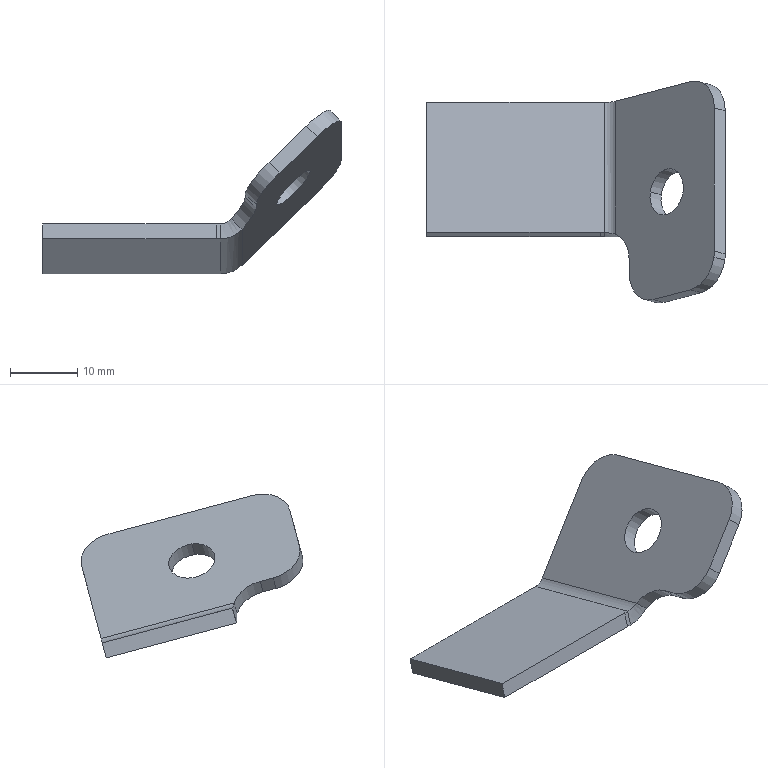Part | SolidWorks | features BaseBody 1, FlatPattern 1, SheetMetal 1, SolidToSheetMetal 1 | 1 solid | 23 faces | box 44.304 x 32.939 x 24.3 mm | volume 2673 mm3 | plane 12 | cylinder 9 | spline 2 | commonest cylinder face diameters 10 x5 7 x2 4.6 x1 9.2 x1
STEP:
#1=CARTESIAN_POINT('',(1147.365,61.574,741.478));
#2=VERTEX_POINT('',#1);
#3=CARTESIAN_POINT('',(1142.501,61.574,736.443));
#4=VERTEX_POINT('',#3);
#5=CARTESIAN_POINT('',(1144.933,61.574,738.961));
#6=DIRECTION('',(0.7071,-0.183,-0.683));
#7=DIRECTION('',(-0.6947,0.,-0.7193));
#8=AXIS2_PLACEMENT_3D('',#5,#6,#7);
#9=CIRCLE('',#8,3.5);
#10=EDGE_CURVE('',#2,#4,#9,.T.);
#11=ORIENTED_EDGE('',*,*,#10,.T.);
#12=CARTESIAN_POINT('',(1140.875,61.995,738.014));
#13=VERTEX_POINT('',#12);
#14=CARTESIAN_POINT('',(1140.875,61.995,738.014));
#15=DIRECTION('',(-0.7071,0.183,0.683));
#16=VECTOR('',#15,1000.);
#17=LINE('',#14,#16);
#18=EDGE_CURVE('',#4,#13,#17,.T.);
#19=ORIENTED_EDGE('',*,*,#18,.T.);
#20=CARTESIAN_POINT('',(1145.738,61.995,743.049));
#21=VERTEX_POINT('',#20);
#22=CARTESIAN_POINT('',(1143.307,61.995,740.532));
#23=DIRECTION('',(0.7071,-0.183,-0.683));
#24=DIRECTION('',(-0.6947,0.,-0.7193));
#25=AXIS2_PLACEMENT_3D('',#22,#23,#24);
#26=CIRCLE('',#25,3.5);
#27=EDGE_CURVE('',#21,#13,#26,.T.);
#28=ORIENTED_EDGE('',*,*,#27,.F.);
#29=CARTESIAN_POINT('',(1145.738,61.995,743.049));
#30=DIRECTION('',(-0.7071,0.183,0.683));
#31=VECTOR('',#30,1000.);
#32=LINE('',#29,#31);
#33=EDGE_CURVE('',#2,#21,#32,.T.);
#34=ORIENTED_EDGE('',*,*,#33,.F.);
#35=EDGE_LOOP('',(#11,#19,#28,#34));
#36=FACE_OUTER_BOUND('',#35,.T.);
#37=CARTESIAN_POINT('',(1143.307,61.995,740.532));
#38=DIRECTION('',(-0.7071,0.183,0.683));
#39=DIRECTION('',(0.6947,0.,0.7193));
#40=AXIS2_PLACEMENT_3D('',#37,#38,#39);
#41=CYLINDRICAL_SURFACE('',#40,3.5);
#42=ADVANCED_FACE('',(#36),#41,.F.);
#43=CARTESIAN_POINT('',(1148.468,47.034,746.517));
#44=VERTEX_POINT('',#43);
#45=CARTESIAN_POINT('',(1151.942,51.864,748.819));
#46=VERTEX_POINT('',#45);
#47=CARTESIAN_POINT('',(1148.468,51.864,745.223));
#48=DIRECTION('',(-0.7071,0.183,0.683));
#49=DIRECTION('',(-0.6947,0.,-0.7193));
#50=AXIS2_PLACEMENT_3D('',#47,#48,#49);
#51=CIRCLE('',#50,5.);
#52=EDGE_CURVE('',#44,#46,#51,.T.);
#53=ORIENTED_EDGE('',*,*,#52,.T.);
#54=CARTESIAN_POINT('',(1150.316,52.285,750.39));
#55=VERTEX_POINT('',#54);
#56=CARTESIAN_POINT('',(1150.316,52.285,750.39));
#57=DIRECTION('',(-0.7071,0.183,0.683));
#58=VECTOR('',#57,1000.);
#59=LINE('',#56,#58);
#60=EDGE_CURVE('',#46,#55,#59,.T.);
#61=ORIENTED_EDGE('',*,*,#60,.T.);
#62=CARTESIAN_POINT('',(1146.842,47.455,748.088));
#63=VERTEX_POINT('',#62);
#64=CARTESIAN_POINT('',(1146.842,52.285,746.794));
#65=DIRECTION('',(-0.7071,0.183,0.683));
#66=DIRECTION('',(-0.6947,0.,-0.7193));
#67=AXIS2_PLACEMENT_3D('',#64,#65,#66);
#68=CIRCLE('',#67,5.);
#69=EDGE_CURVE('',#63,#55,#68,.T.);
#70=ORIENTED_EDGE('',*,*,#69,.F.);
#71=CARTESIAN_POINT('',(1146.842,47.455,748.088));
#72=DIRECTION('',(-0.7071,0.183,0.683));
#73=VECTOR('',#72,1000.);
#74=LINE('',#71,#73);
#75=EDGE_CURVE('',#44,#63,#74,.T.);
#76=ORIENTED_EDGE('',*,*,#75,.F.);
#77=EDGE_LOOP('',(#53,#61,#70,#76));
#78=FACE_OUTER_BOUND('',#77,.T.);
#79=CARTESIAN_POINT('',(1146.842,52.285,746.794));
#80=DIRECTION('',(-0.7071,0.183,0.683));
#81=DIRECTION('',(0.6947,0.,0.7193));
#82=AXIS2_PLACEMENT_3D('',#79,#80,#81);
#83=CYLINDRICAL_SURFACE('',#82,5.);
#84=ADVANCED_FACE('',(#78),#83,.T.);
#85=CARTESIAN_POINT('',(1139.381,51.444,735.927));
#86=VERTEX_POINT('',#85);
#87=CARTESIAN_POINT('',(1137.755,51.865,737.498));
#88=VERTEX_POINT('',#87);
#89=CARTESIAN_POINT('',(1137.755,51.865,737.498));
#90=DIRECTION('',(-0.7071,0.183,0.683));
#91=VECTOR('',#90,1000.);
#92=LINE('',#89,#91);
#93=EDGE_CURVE('',#86,#88,#92,.T.);
#94=ORIENTED_EDGE('',*,*,#93,.F.);
#95=CARTESIAN_POINT('',(1139.381,49.512,736.445));
#96=VERTEX_POINT('',#95);
#97=CARTESIAN_POINT('',(1139.381,51.444,735.927));
#98=DIRECTION('',(-0.000000007,-0.9659,0.2588));
#99=VECTOR('',#98,1000.);
#100=LINE('',#97,#99);
#101=EDGE_CURVE('',#86,#96,#100,.T.);
#102=ORIENTED_EDGE('',*,*,#101,.T.);
#103=CARTESIAN_POINT('',(1137.755,49.933,738.016));
#104=VERTEX_POINT('',#103);
#105=CARTESIAN_POINT('',(1137.755,49.933,738.016));
#106=DIRECTION('',(-0.7071,0.183,0.683));
#107=VECTOR('',#106,1000.);
#108=LINE('',#105,#107);
#109=EDGE_CURVE('',#96,#104,#108,.T.);
#110=ORIENTED_EDGE('',*,*,#109,.T.);
#111=CARTESIAN_POINT('',(1137.755,51.865,737.498));
#112=DIRECTION('',(-0.000000007,-0.9659,0.2588));
#113=VECTOR('',#112,1000.);
#114=LINE('',#111,#113);
#115=EDGE_CURVE('',#88,#104,#114,.T.);
#116=ORIENTED_EDGE('',*,*,#115,.F.);
#117=EDGE_LOOP('',(#94,#102,#110,#116));
#118=FACE_OUTER_BOUND('',#117,.T.);
#119=CARTESIAN_POINT('',(1137.755,51.865,737.498));
#120=DIRECTION('',(-0.7071,-0.183,-0.683));
#121=DIRECTION('',(-0.000000007,-0.9659,0.2588));
#122=AXIS2_PLACEMENT_3D('',#119,#120,#121);
#123=PLANE('',#122);
#124=ADVANCED_FACE('',(#118),#123,.T.);
#125=ORIENTED_EDGE('',*,*,#109,.F.);
#126=CARTESIAN_POINT('',(1142.917,45.597,741.154));
#127=VERTEX_POINT('',#126);
#128=CARTESIAN_POINT('',(1142.917,50.427,739.86));
#129=DIRECTION('',(-0.7071,0.183,0.683));
#130=DIRECTION('',(0.6947,0.,0.7193));
#131=AXIS2_PLACEMENT_3D('',#128,#129,#130);
#132=CIRCLE('',#131,5.);
#133=EDGE_CURVE('',#96,#127,#132,.T.);
#134=ORIENTED_EDGE('',*,*,#133,.T.);
#135=CARTESIAN_POINT('',(1141.29,46.018,742.725));
#136=VERTEX_POINT('',#135);
#137=CARTESIAN_POINT('',(1141.29,46.018,742.725));
#138=DIRECTION('',(-0.7071,0.183,0.683));
#139=VECTOR('',#138,1000.);
#140=LINE('',#137,#139);
#141=EDGE_CURVE('',#127,#136,#140,.T.);
#142=ORIENTED_EDGE('',*,*,#141,.T.);
#143=CARTESIAN_POINT('',(1141.29,50.848,741.431));
#144=DIRECTION('',(-0.7071,0.183,0.683));
#145=DIRECTION('',(0.6947,0.,0.7193));
#146=AXIS2_PLACEMENT_3D('',#143,#144,#145);
#147=CIRCLE('',#146,5.);
#148=EDGE_CURVE('',#104,#136,#147,.T.);
#149=ORIENTED_EDGE('',*,*,#148,.F.);
#150=EDGE_LOOP('',(#125,#134,#142,#149));
#151=FACE_OUTER_BOUND('',#150,.T.);
#152=CARTESIAN_POINT('',(1141.29,50.848,741.431));
#153=DIRECTION('',(-0.7071,0.183,0.683));
#154=DIRECTION('',(0.6947,0.,0.7193));
#155=AXIS2_PLACEMENT_3D('',#152,#153,#154);
#156=CYLINDRICAL_SURFACE('',#155,5.);
#157=ADVANCED_FACE('',(#151),#156,.T.);
#158=ORIENTED_EDGE('',*,*,#141,.F.);
#159=CARTESIAN_POINT('',(1142.917,45.597,741.154));
#160=DIRECTION('',(0.7071,0.183,0.683));
#161=VECTOR('',#160,1000.);
#162=LINE('',#159,#161);
#163=EDGE_CURVE('',#127,#44,#162,.T.);
#164=ORIENTED_EDGE('',*,*,#163,.T.);
#165=ORIENTED_EDGE('',*,*,#75,.T.);
#166=CARTESIAN_POINT('',(1141.29,46.018,742.725));
#167=DIRECTION('',(0.7071,0.183,0.683));
#168=VECTOR('',#167,1000.);
#169=LINE('',#166,#168);
#170=EDGE_CURVE('',#136,#63,#169,.T.);
#171=ORIENTED_EDGE('',*,*,#170,.F.);
#172=EDGE_LOOP('',(#158,#164,#165,#171));
#173=FACE_OUTER_BOUND('',#172,.T.);
#174=CARTESIAN_POINT('',(1141.29,46.018,742.725));
#175=DIRECTION('',(0.000000002,-0.9659,0.2588));
#176=DIRECTION('',(0.7071,0.183,0.683));
#177=AXIS2_PLACEMENT_3D('',#174,#175,#176);
#178=PLANE('',#177);
#179=ADVANCED_FACE('',(#173),#178,.T.);
#180=ORIENTED_EDGE('',*,*,#60,.F.);
#181=CARTESIAN_POINT('',(1152.004,52.779,748.638));
#182=VERTEX_POINT('',#181);
#183=CARTESIAN_POINT('',(1148.468,51.864,745.223));
#184=DIRECTION('',(-0.7071,0.183,0.683));
#185=DIRECTION('',(-0.6947,0.,-0.7193));
#186=AXIS2_PLACEMENT_3D('',#183,#184,#185);
#187=CIRCLE('',#186,5.);
#188=EDGE_CURVE('',#46,#182,#187,.T.);
#189=ORIENTED_EDGE('',*,*,#188,.T.);
#190=CARTESIAN_POINT('',(1150.378,53.2,750.209));
#191=VERTEX_POINT('',#190);
#192=CARTESIAN_POINT('',(1150.378,53.2,750.209));
#193=DIRECTION('',(-0.7071,0.183,0.683));
#194=VECTOR('',#193,1000.);
#195=LINE('',#192,#194);
#196=EDGE_CURVE('',#182,#191,#195,.T.);
#197=ORIENTED_EDGE('',*,*,#196,.T.);
#198=CARTESIAN_POINT('',(1146.842,52.285,746.794));
#199=DIRECTION('',(-0.7071,0.183,0.683));
#200=DIRECTION('',(-0.6947,0.,-0.7193));
#201=AXIS2_PLACEMENT_3D('',#198,#199,#200);
#202=CIRCLE('',#201,5.);
#203=EDGE_CURVE('',#55,#191,#202,.T.);
#204=ORIENTED_EDGE('',*,*,#203,.F.);
#205=EDGE_LOOP('',(#180,#189,#197,#204));
#206=FACE_OUTER_BOUND('',#205,.T.);
#207=CARTESIAN_POINT('',(1146.842,52.285,746.794));
#208=DIRECTION('',(-0.7071,0.183,0.683));
#209=DIRECTION('',(0.6947,0.,0.7193));
#210=AXIS2_PLACEMENT_3D('',#207,#208,#209);
#211=CYLINDRICAL_SURFACE('',#210,5.);
#212=ADVANCED_FACE('',(#206),#211,.T.);
#213=ORIENTED_EDGE('',*,*,#196,.F.);
#214=CARTESIAN_POINT('',(1152.004,74.029,742.944));
#215=VERTEX_POINT('',#214);
#216=CARTESIAN_POINT('',(1152.004,52.779,748.638));
#217=DIRECTION('',(0.,0.9659,-0.2588));
#218=VECTOR('',#217,1000.);
#219=LINE('',#216,#218);
#220=EDGE_CURVE('',#182,#215,#219,.T.);
#221=ORIENTED_EDGE('',*,*,#220,.T.);
#222=CARTESIAN_POINT('',(1150.378,74.45,744.515));
#223=VERTEX_POINT('',#222);
#224=CARTESIAN_POINT('',(1150.378,74.45,744.515));
#225=DIRECTION('',(-0.7071,0.183,0.683));
#226=VECTOR('',#225,1000.);
#227=LINE('',#224,#226);
#228=EDGE_CURVE('',#215,#223,#227,.T.);
#229=ORIENTED_EDGE('',*,*,#228,.T.);
#230=CARTESIAN_POINT('',(1150.378,53.2,750.209));
#231=DIRECTION('',(0.,0.9659,-0.2588));
#232=VECTOR('',#231,1000.);
#233=LINE('',#230,#232);
#234=EDGE_CURVE('',#191,#223,#233,.T.);
#235=ORIENTED_EDGE('',*,*,#234,.F.);
#236=EDGE_LOOP('',(#213,#221,#229,#235));
#237=FACE_OUTER_BOUND('',#236,.T.);
#238=CARTESIAN_POINT('',(1150.378,53.2,750.209));
#239=DIRECTION('',(0.7071,0.183,0.683));
#240=DIRECTION('',(0.,0.9659,-0.2588));
#241=AXIS2_PLACEMENT_3D('',#238,#239,#240);
#242=PLANE('',#241);
#243=ADVANCED_FACE('',(#237),#242,.T.);
#244=ORIENTED_EDGE('',*,*,#228,.F.);
#245=CARTESIAN_POINT('',(1148.468,77.944,738.235));
#246=VERTEX_POINT('',#245);
#247=CARTESIAN_POINT('',(1148.468,73.114,739.529));
#248=DIRECTION('',(-0.7071,0.183,0.683));
#249=DIRECTION('',(-0.6947,0.,-0.7193));
#250=AXIS2_PLACEMENT_3D('',#247,#248,#249);
#251=CIRCLE('',#250,5.);
#252=EDGE_CURVE('',#215,#246,#251,.T.);
#253=ORIENTED_EDGE('',*,*,#252,.T.);
#254=CARTESIAN_POINT('',(1146.842,78.365,739.805));
#255=VERTEX_POINT('',#254);
#256=CARTESIAN_POINT('',(1146.842,78.365,739.805));
#257=DIRECTION('',(-0.7071,0.183,0.683));
#258=VECTOR('',#257,1000.);
#259=LINE('',#256,#258);
#260=EDGE_CURVE('',#246,#255,#259,.T.);
#261=ORIENTED_EDGE('',*,*,#260,.T.);
#262=CARTESIAN_POINT('',(1146.842,73.535,741.1));
#263=DIRECTION('',(-0.7071,0.183,0.683));
#264=DIRECTION('',(-0.6947,0.,-0.7193));
#265=AXIS2_PLACEMENT_3D('',#262,#263,#264);
#266=CIRCLE('',#265,5.);
#267=EDGE_CURVE('',#223,#255,#266,.T.);
#268=ORIENTED_EDGE('',*,*,#267,.F.);
#269=EDGE_LOOP('',(#244,#253,#261,#268));
#270=FACE_OUTER_BOUND('',#269,.T.);
#271=CARTESIAN_POINT('',(1146.842,73.535,741.1));
#272=DIRECTION('',(-0.7071,0.183,0.683));
#273=DIRECTION('',(0.6947,0.,0.7193));
#274=AXIS2_PLACEMENT_3D('',#271,#272,#273);
#275=CYLINDRICAL_SURFACE('',#274,5.);
#276=ADVANCED_FACE('',(#270),#275,.T.);
#277=ORIENTED_EDGE('',*,*,#260,.F.);
#278=CARTESIAN_POINT('',(1137.3,75.053,727.447));
#279=VERTEX_POINT('',#278);
#280=CARTESIAN_POINT('',(1148.468,77.944,738.235));
#281=DIRECTION('',(-0.7071,-0.183,-0.683));
#282=VECTOR('',#281,1000.);
#283=LINE('',#280,#282);
#284=EDGE_CURVE('',#246,#279,#283,.T.);
#285=ORIENTED_EDGE('',*,*,#284,.T.);
#286=CARTESIAN_POINT('',(1135.674,75.474,729.018));
#287=VERTEX_POINT('',#286);
#288=CARTESIAN_POINT('',(1135.674,75.474,729.018));
#289=DIRECTION('',(-0.7071,0.183,0.683));
#290=VECTOR('',#289,1000.);
#291=LINE('',#288,#290);
#292=EDGE_CURVE('',#279,#287,#291,.T.);
#293=ORIENTED_EDGE('',*,*,#292,.T.);
#294=CARTESIAN_POINT('',(1146.842,78.365,739.805));
#295=DIRECTION('',(-0.7071,-0.183,-0.683));
#296=VECTOR('',#295,1000.);
#297=LINE('',#294,#296);
#298=EDGE_CURVE('',#255,#287,#297,.T.);
#299=ORIENTED_EDGE('',*,*,#298,.F.);
#300=EDGE_LOOP('',(#277,#285,#293,#299));
#301=FACE_OUTER_BOUND('',#300,.T.);
#302=CARTESIAN_POINT('',(1146.842,78.365,739.805));
#303=DIRECTION('',(0.,0.9659,-0.2588));
#304=DIRECTION('',(-0.7071,-0.183,-0.683));
#305=AXIS2_PLACEMENT_3D('',#302,#303,#304);
#306=PLANE('',#305);
#307=ADVANCED_FACE('',(#301),#306,.T.);
#308=ORIENTED_EDGE('',*,*,#292,.F.);
#309=CARTESIAN_POINT('',(1134.047,74.705,726.145));
#310=VERTEX_POINT('',#309);
#311=CARTESIAN_POINT('',(1134.047,75.895,730.588));
#312=DIRECTION('',(0.,0.9659,-0.2588));
#313=DIRECTION('',(0.,0.2588,0.9659));
#314=AXIS2_PLACEMENT_3D('',#311,#312,#313);
#315=CIRCLE('',#314,4.6);
#316=EDGE_CURVE('',#279,#310,#315,.T.);
#317=ORIENTED_EDGE('',*,*,#316,.T.);
#318=CARTESIAN_POINT('',(1134.047,75.3,728.367));
#319=VERTEX_POINT('',#318);
#320=CARTESIAN_POINT('',(1134.047,75.3,728.367));
#321=DIRECTION('',(0.,0.2588,0.9659));
#322=VECTOR('',#321,1000.);
#323=LINE('',#320,#322);
#324=EDGE_CURVE('',#310,#319,#323,.T.);
#325=ORIENTED_EDGE('',*,*,#324,.T.);
#326=CARTESIAN_POINT('',(1134.047,75.895,730.588));
#327=DIRECTION('',(0.,0.9659,-0.2588));
#328=DIRECTION('',(0.,0.2588,0.9659));
#329=AXIS2_PLACEMENT_3D('',#326,#327,#328);
#330=CIRCLE('',#329,2.3);
#331=EDGE_CURVE('',#287,#319,#330,.T.);
#332=ORIENTED_EDGE('',*,*,#331,.F.);
#333=EDGE_LOOP('',(#308,#317,#325,#332));
#334=FACE_OUTER_BOUND('',#333,.T.);
#335=CARTESIAN_POINT('',(1134.047,75.895,730.588));
#336=DIRECTION('',(0.,-0.9659,0.2588));
#337=DIRECTION('',(0.,-0.2588,-0.9659));
#338=AXIS2_PLACEMENT_3D('',#335,#336,#337);
#339=PLANE('',#338);
#340=ADVANCED_FACE('',(#334),#339,.F.);
#341=ORIENTED_EDGE('',*,*,#324,.F.);
#342=CARTESIAN_POINT('',(1107.7,74.705,726.145));
#343=VERTEX_POINT('',#342);
#344=CARTESIAN_POINT('',(1134.047,74.705,726.145));
#345=DIRECTION('',(1.,0.,0.));
#346=VECTOR('',#345,1000.);
#347=LINE('',#344,#346);
#348=EDGE_CURVE('',#343,#310,#347,.T.);
#349=ORIENTED_EDGE('',*,*,#348,.F.);
#350=CARTESIAN_POINT('',(1107.7,75.3,728.367));
#351=VERTEX_POINT('',#350);
#352=CARTESIAN_POINT('',(1107.7,75.3,728.367));
#353=DIRECTION('',(0.,0.2588,0.9659));
#354=VECTOR('',#353,1000.);
#355=LINE('',#352,#354);
#356=EDGE_CURVE('',#343,#351,#355,.T.);
#357=ORIENTED_EDGE('',*,*,#356,.T.);
#358=CARTESIAN_POINT('',(1120.874,75.3,728.367));
#359=DIRECTION('',(1.,0.,0.));
#360=VECTOR('',#359,1000.);
#361=LINE('',#358,#360);
#362=EDGE_CURVE('',#351,#319,#361,.T.);
#363=ORIENTED_EDGE('',*,*,#362,.T.);
#364=EDGE_LOOP('',(#341,#349,#357,#363));
#365=FACE_OUTER_BOUND('',#364,.T.);
#366=CARTESIAN_POINT('',(1120.874,75.3,728.367));
#367=DIRECTION('',(0.,0.9659,-0.2588));
#368=DIRECTION('',(1.,0.,0.));
#369=AXIS2_PLACEMENT_3D('',#366,#367,#368);
#370=PLANE('',#369);
#371=ADVANCED_FACE('',(#365),#370,.T.);
#372=ORIENTED_EDGE('',*,*,#356,.F.);
#373=CARTESIAN_POINT('',(1107.7,55.386,731.322));
#374=VERTEX_POINT('',#373);
#375=CARTESIAN_POINT('',(1107.7,74.705,726.145));
#376=DIRECTION('',(0.,0.9659,-0.2588));
#377=VECTOR('',#376,1000.);
#378=LINE('',#375,#377);
#379=EDGE_CURVE('',#374,#343,#378,.T.);
#380=ORIENTED_EDGE('',*,*,#379,.F.);
#381=CARTESIAN_POINT('',(1107.7,55.981,733.543));
#382=VERTEX_POINT('',#381);
#383=CARTESIAN_POINT('',(1107.7,55.981,733.543));
#384=DIRECTION('',(0.,0.2588,0.9659));
#385=VECTOR('',#384,1000.);
#386=LINE('',#383,#385);
#387=EDGE_CURVE('',#374,#382,#386,.T.);
#388=ORIENTED_EDGE('',*,*,#387,.T.);
#389=CARTESIAN_POINT('',(1107.7,65.574,730.973));
#390=DIRECTION('',(0.,0.9659,-0.2588));
#391=VECTOR('',#390,1000.);
#392=LINE('',#389,#391);
#393=EDGE_CURVE('',#382,#351,#392,.T.);
#394=ORIENTED_EDGE('',*,*,#393,.T.);
#395=EDGE_LOOP('',(#372,#380,#388,#394));
#396=FACE_OUTER_BOUND('',#395,.T.);
#397=CARTESIAN_POINT('',(1107.7,65.574,730.973));
#398=DIRECTION('',(-1.,0.,0.));
#399=DIRECTION('',(0.,0.9659,-0.2588));
#400=AXIS2_PLACEMENT_3D('',#397,#398,#399);
#401=PLANE('',#400);
#402=ADVANCED_FACE('',(#396),#401,.T.);
#403=ORIENTED_EDGE('',*,*,#387,.F.);
#404=CARTESIAN_POINT('',(1133.438,55.386,731.322));
#405=VERTEX_POINT('',#404);
#406=CARTESIAN_POINT('',(1134.047,55.386,731.322));
#407=DIRECTION('',(-1.,0.,0.));
#408=VECTOR('',#407,1000.);
#409=LINE('',#406,#408);
#410=EDGE_CURVE('',#405,#374,#409,.T.);
#411=ORIENTED_EDGE('',*,*,#410,.F.);
#412=CARTESIAN_POINT('',(1133.438,55.981,733.543));
#413=VERTEX_POINT('',#412);
#414=CARTESIAN_POINT('',(1133.438,55.981,733.543));
#415=DIRECTION('',(0.,0.2588,0.9659));
#416=VECTOR('',#415,1000.);
#417=LINE('',#414,#416);
#418=EDGE_CURVE('',#405,#413,#417,.T.);
#419=ORIENTED_EDGE('',*,*,#418,.T.);
#420=CARTESIAN_POINT('',(1120.874,55.981,733.543));
#421=DIRECTION('',(-1.,0.,0.));
#422=VECTOR('',#421,1000.);
#423=LINE('',#420,#422);
#424=EDGE_CURVE('',#413,#382,#423,.T.);
#425=ORIENTED_EDGE('',*,*,#424,.T.);
#426=EDGE_LOOP('',(#403,#411,#419,#425));
#427=FACE_OUTER_BOUND('',#426,.T.);
#428=CARTESIAN_POINT('',(1120.874,55.981,733.543));
#429=DIRECTION('',(0.,-0.9659,0.2588));
#430=DIRECTION('',(-1.,0.,0.));
#431=AXIS2_PLACEMENT_3D('',#428,#429,#430);
#432=PLANE('',#431);
#433=ADVANCED_FACE('',(#427),#432,.T.);
#434=ORIENTED_EDGE('',*,*,#418,.F.);
#435=CARTESIAN_POINT('',(1134.047,55.368,731.326));
#436=VERTEX_POINT('',#435);
#437=CARTESIAN_POINT('',(1134.047,55.368,731.326));
#438=CARTESIAN_POINT('',(1133.845,55.38,731.323));
#439=CARTESIAN_POINT('',(1133.642,55.386,731.322));
#440=CARTESIAN_POINT('',(1133.438,55.386,731.322));
#441=(BOUNDED_CURVE()B_SPLINE_CURVE(3,(#437,#438,#439,#440),.UNSPECIFIED.,.F.,.F.)B_SPLINE_CURVE_WITH_KNOTS((4,4),(1.485,1.571),.UNSPECIFIED.)CURVE()GEOMETRIC_REPRESENTATION_ITEM()RATIONAL_B_SPLINE_CURVE((1.,0.9994,0.9994,1.))REPRESENTATION_ITEM(''));
#442=EDGE_CURVE('',#436,#405,#441,.T.);
#443=ORIENTED_EDGE('',*,*,#442,.F.);
#444=CARTESIAN_POINT('',(1134.047,55.964,733.548));
#445=VERTEX_POINT('',#444);
#446=CARTESIAN_POINT('',(1134.047,55.368,731.326));
#447=CARTESIAN_POINT('',(1134.047,55.964,733.548));
#448=B_SPLINE_CURVE_WITH_KNOTS('',1,(#446,#447),.UNSPECIFIED.,.F.,.F.,(2,2),(0.,1.),.UNSPECIFIED.);
#449=EDGE_CURVE('',#436,#445,#448,.T.);
#450=ORIENTED_EDGE('',*,*,#449,.T.);
#451=CARTESIAN_POINT('',(1134.047,55.964,733.548));
#452=CARTESIAN_POINT('',(1133.845,55.975,733.545));
#453=CARTESIAN_POINT('',(1133.642,55.981,733.543));
#454=CARTESIAN_POINT('',(1133.438,55.981,733.543));
#455=(BOUNDED_CURVE()B_SPLINE_CURVE(3,(#451,#452,#453,#454),.UNSPECIFIED.,.F.,.F.)B_SPLINE_CURVE_WITH_KNOTS((4,4),(1.485,1.571),.UNSPECIFIED.)CURVE()GEOMETRIC_REPRESENTATION_ITEM()RATIONAL_B_SPLINE_CURVE((1.,0.9994,0.9994,1.))REPRESENTATION_ITEM(''));
#456=EDGE_CURVE('',#445,#413,#455,.T.);
#457=ORIENTED_EDGE('',*,*,#456,.T.);
#458=EDGE_LOOP('',(#434,#443,#450,#457));
#459=FACE_OUTER_BOUND('',#458,.T.);
#460=CARTESIAN_POINT('',(1134.047,55.964,733.548));
#461=CARTESIAN_POINT('',(1134.047,55.368,731.326));
#462=CARTESIAN_POINT('',(1133.845,55.975,733.545));
#463=CARTESIAN_POINT('',(1133.845,55.38,731.323));
#464=CARTESIAN_POINT('',(1133.642,55.981,733.543));
#465=CARTESIAN_POINT('',(1133.642,55.386,731.322));
#466=CARTESIAN_POINT('',(1133.438,55.981,733.543));
#467=CARTESIAN_POINT('',(1133.438,55.386,731.322));
#468=(BOUNDED_SURFACE()B_SPLINE_SURFACE(3,1,((#460,#461),(#462,#463),(#464,#465),(#466,#467)),.UNSPECIFIED.,.F.,.F.,.F.)B_SPLINE_SURFACE_WITH_KNOTS((4,4),(2,2),(0.,1.),(0.,1.),.UNSPECIFIED.)GEOMETRIC_REPRESENTATION_ITEM()RATIONAL_B_SPLINE_SURFACE(((1.,1.),(0.9994,0.9994),(0.9994,0.9994),(1.,1.)))REPRESENTATION_ITEM('')SURFACE());
#469=ADVANCED_FACE('',(#459),#468,.F.);
#470=ORIENTED_EDGE('',*,*,#449,.F.);
#471=CARTESIAN_POINT('',(1137.3,55.307,732.738));
#472=VERTEX_POINT('',#471);
#473=CARTESIAN_POINT('',(1134.047,55.368,731.326));
#474=CARTESIAN_POINT('',(1134.36,55.359,731.329));
#475=CARTESIAN_POINT('',(1134.667,55.354,731.363));
#476=CARTESIAN_POINT('',(1135.268,55.346,731.492));
#477=CARTESIAN_POINT('',(1135.566,55.344,731.589));
#478=CARTESIAN_POINT('',(1136.122,55.338,731.835));
#479=CARTESIAN_POINT('',(1136.384,55.335,731.984));
#480=CARTESIAN_POINT('',(1136.873,55.324,732.33));
#481=CARTESIAN_POINT('',(1137.099,55.317,732.527));
#482=CARTESIAN_POINT('',(1137.3,55.307,732.738));
#483=B_SPLINE_CURVE_WITH_KNOTS('',3,(#473,#474,#475,#476,#477,#478,#479,#480,#481,#482),.UNSPECIFIED.,.F.,.F.,(4,2,2,2,4),(0.,0.25,0.5,0.75,1.),.UNSPECIFIED.);
#484=EDGE_CURVE('',#436,#472,#483,.T.);
#485=ORIENTED_EDGE('',*,*,#484,.T.);
#486=CARTESIAN_POINT('',(1135.674,55.728,734.308));
#487=VERTEX_POINT('',#486);
#488=CARTESIAN_POINT('',(1137.3,55.307,732.738));
#489=CARTESIAN_POINT('',(1135.674,55.728,734.308));
#490=B_SPLINE_CURVE_WITH_KNOTS('',1,(#488,#489),.UNSPECIFIED.,.F.,.F.,(2,2),(0.,1.),.UNSPECIFIED.);
#491=EDGE_CURVE('',#472,#487,#490,.T.);
#492=ORIENTED_EDGE('',*,*,#491,.T.);
#493=CARTESIAN_POINT('',(1134.047,55.964,733.548));
#494=CARTESIAN_POINT('',(1134.215,55.954,733.551));
#495=CARTESIAN_POINT('',(1134.376,55.943,733.573));
#496=CARTESIAN_POINT('',(1134.602,55.925,733.627));
#497=CARTESIAN_POINT('',(1134.675,55.919,733.649));
#498=CARTESIAN_POINT('',(1134.779,55.908,733.686));
#499=CARTESIAN_POINT('',(1134.831,55.903,733.706));
#500=CARTESIAN_POINT('',(1134.881,55.897,733.728));
#501=CARTESIAN_POINT('',(1134.913,55.893,733.742));
#502=CARTESIAN_POINT('',(1134.928,55.891,733.749));
#503=CARTESIAN_POINT('',(1135.223,55.853,733.889));
#504=CARTESIAN_POINT('',(1135.47,55.801,734.079));
#505=CARTESIAN_POINT('',(1135.674,55.728,734.308));
#506=B_SPLINE_CURVE_WITH_KNOTS('',3,(#493,#494,#495,#496,#497,#498,#499,#500,#501,#502,#503,#504,#505),.UNSPECIFIED.,.F.,.F.,(4,2,2,1,2,2,4),(0.,0.25,0.375,0.4375,0.4687,0.5,1.),.UNSPECIFIED.);
#507=EDGE_CURVE('',#445,#487,#506,.T.);
#508=ORIENTED_EDGE('',*,*,#507,.F.);
#509=EDGE_LOOP('',(#470,#485,#492,#508));
#510=FACE_OUTER_BOUND('',#509,.T.);
#511=CARTESIAN_POINT('',(1134.047,55.368,731.326));
#512=CARTESIAN_POINT('',(1134.36,55.359,731.329));
#513=CARTESIAN_POINT('',(1134.667,55.354,731.363));
#514=CARTESIAN_POINT('',(1135.268,55.346,731.492));
#515=CARTESIAN_POINT('',(1135.566,55.344,731.589));
#516=CARTESIAN_POINT('',(1136.122,55.338,731.835));
#517=CARTESIAN_POINT('',(1136.384,55.335,731.984));
#518=CARTESIAN_POINT('',(1136.873,55.324,732.33));
#519=CARTESIAN_POINT('',(1137.099,55.317,732.527));
#520=CARTESIAN_POINT('',(1137.3,55.307,732.738));
#521=CARTESIAN_POINT('',(1134.047,55.964,733.548));
#522=CARTESIAN_POINT('',(1134.204,55.954,733.551));
#523=CARTESIAN_POINT('',(1134.357,55.945,733.569));
#524=CARTESIAN_POINT('',(1134.658,55.921,733.639));
#525=CARTESIAN_POINT('',(1134.806,55.907,733.691));
#526=CARTESIAN_POINT('',(1135.085,55.871,733.823));
#527=CARTESIAN_POINT('',(1135.215,55.849,733.903));
#528=CARTESIAN_POINT('',(1135.46,55.796,734.089));
#529=CARTESIAN_POINT('',(1135.573,55.764,734.195));
#530=CARTESIAN_POINT('',(1135.674,55.728,734.308));
#531=B_SPLINE_SURFACE_WITH_KNOTS('',1,3,((#511,#512,#513,#514,#515,#516,#517,#518,#519,#520),(#521,#522,#523,#524,#525,#526,#527,#528,#529,#530)),.UNSPECIFIED.,.F.,.F.,.F.,(2,2),(4,2,2,2,4),(0.,1.),(0.,0.0004637,0.0009275,0.001391,0.001855),.UNSPECIFIED.);
#532=ADVANCED_FACE('',(#510),#531,.F.);
#533=ORIENTED_EDGE('',*,*,#18,.F.);
#534=CARTESIAN_POINT('',(1144.933,61.574,738.961));
#535=DIRECTION('',(0.7071,-0.183,-0.683));
#536=DIRECTION('',(-0.6947,0.,-0.7193));
#537=AXIS2_PLACEMENT_3D('',#534,#535,#536);
#538=CIRCLE('',#537,3.5);
#539=EDGE_CURVE('',#4,#2,#538,.T.);
#540=ORIENTED_EDGE('',*,*,#539,.T.);
#541=ORIENTED_EDGE('',*,*,#33,.T.);
#542=CARTESIAN_POINT('',(1143.307,61.995,740.532));
#543=DIRECTION('',(0.7071,-0.183,-0.683));
#544=DIRECTION('',(-0.6947,0.,-0.7193));
#545=AXIS2_PLACEMENT_3D('',#542,#543,#544);
#546=CIRCLE('',#545,3.5);
#547=EDGE_CURVE('',#13,#21,#546,.T.);
#548=ORIENTED_EDGE('',*,*,#547,.F.);
#549=EDGE_LOOP('',(#533,#540,#541,#548));
#550=FACE_OUTER_BOUND('',#549,.T.);
#551=CARTESIAN_POINT('',(1143.307,61.995,740.532));
#552=DIRECTION('',(-0.7071,0.183,0.683));
#553=DIRECTION('',(0.6947,0.,0.7193));
#554=AXIS2_PLACEMENT_3D('',#551,#552,#553);
#555=CYLINDRICAL_SURFACE('',#554,3.5);
#556=ADVANCED_FACE('',(#550),#555,.F.);
#557=CARTESIAN_POINT('',(1135.846,50.529,732.512));
#558=DIRECTION('',(0.7071,-0.183,-0.683));
#559=DIRECTION('',(-0.6947,0.,-0.7193));
#560=AXIS2_PLACEMENT_3D('',#557,#558,#559);
#561=CIRCLE('',#560,5.);
#562=EDGE_CURVE('',#472,#86,#561,.T.);
#563=ORIENTED_EDGE('',*,*,#562,.T.);
#564=ORIENTED_EDGE('',*,*,#93,.T.);
#565=CARTESIAN_POINT('',(1134.219,50.95,734.083));
#566=DIRECTION('',(0.7071,-0.183,-0.683));
#567=DIRECTION('',(-0.6947,0.,-0.7193));
#568=AXIS2_PLACEMENT_3D('',#565,#566,#567);
#569=CIRCLE('',#568,5.);
#570=EDGE_CURVE('',#487,#88,#569,.T.);
#571=ORIENTED_EDGE('',*,*,#570,.F.);
#572=ORIENTED_EDGE('',*,*,#491,.F.);
#573=EDGE_LOOP('',(#563,#564,#571,#572));
#574=FACE_OUTER_BOUND('',#573,.T.);
#575=CARTESIAN_POINT('',(1134.219,50.95,734.083));
#576=DIRECTION('',(-0.7071,0.183,0.683));
#577=DIRECTION('',(0.6947,0.,0.7193));
#578=AXIS2_PLACEMENT_3D('',#575,#576,#577);
#579=CYLINDRICAL_SURFACE('',#578,5.);
#580=ADVANCED_FACE('',(#574),#579,.F.);
#581=ORIENTED_EDGE('',*,*,#507,.T.);
#582=CARTESIAN_POINT('',(1135.674,65.542,731.679));
#583=DIRECTION('',(0.,0.9659,-0.2588));
#584=VECTOR('',#583,1000.);
#585=LINE('',#582,#584);
#586=EDGE_CURVE('',#487,#287,#585,.T.);
#587=ORIENTED_EDGE('',*,*,#586,.T.);
#588=ORIENTED_EDGE('',*,*,#331,.T.);
#589=CARTESIAN_POINT('',(1134.047,65.574,730.973));
#590=DIRECTION('',(0.,-0.9659,0.2588));
#591=VECTOR('',#590,1000.);
#592=LINE('',#589,#591);
#593=EDGE_CURVE('',#319,#445,#592,.T.);
#594=ORIENTED_EDGE('',*,*,#593,.T.);
#595=EDGE_LOOP('',(#581,#587,#588,#594));
#596=FACE_OUTER_BOUND('',#595,.T.);
#597=CARTESIAN_POINT('',(1134.047,56.031,735.911));
#598=DIRECTION('',(0.,0.9659,-0.2588));
#599=DIRECTION('',(0.,0.2588,0.9659));
#600=AXIS2_PLACEMENT_3D('',#597,#598,#599);
#601=CYLINDRICAL_SURFACE('',#600,2.3);
#602=ADVANCED_FACE('',(#596),#601,.F.);
#603=ORIENTED_EDGE('',*,*,#593,.F.);
#604=ORIENTED_EDGE('',*,*,#362,.F.);
#605=ORIENTED_EDGE('',*,*,#393,.F.);
#606=ORIENTED_EDGE('',*,*,#424,.F.);
#607=ORIENTED_EDGE('',*,*,#456,.F.);
#608=EDGE_LOOP('',(#603,#604,#605,#606,#607));
#609=FACE_OUTER_BOUND('',#608,.T.);
#610=CARTESIAN_POINT('',(1134.047,75.3,728.367));
#611=DIRECTION('',(0.,-0.2588,-0.9659));
#612=DIRECTION('',(0.,-0.9659,0.2588));
#613=AXIS2_PLACEMENT_3D('',#610,#611,#612);
#614=PLANE('',#613);
#615=ADVANCED_FACE('',(#609),#614,.F.);
#616=ORIENTED_EDGE('',*,*,#27,.T.);
#617=ORIENTED_EDGE('',*,*,#547,.T.);
#618=EDGE_LOOP('',(#616,#617));
#619=FACE_BOUND('',#618,.T.);
#620=ORIENTED_EDGE('',*,*,#570,.T.);
#621=ORIENTED_EDGE('',*,*,#115,.T.);
#622=ORIENTED_EDGE('',*,*,#148,.T.);
#623=ORIENTED_EDGE('',*,*,#170,.T.);
#624=ORIENTED_EDGE('',*,*,#69,.T.);
#625=ORIENTED_EDGE('',*,*,#203,.T.);
#626=ORIENTED_EDGE('',*,*,#234,.T.);
#627=ORIENTED_EDGE('',*,*,#267,.T.);
#628=ORIENTED_EDGE('',*,*,#298,.T.);
#629=ORIENTED_EDGE('',*,*,#586,.F.);
#630=EDGE_LOOP('',(#620,#621,#622,#623,#624,#625,#626,#627,#628,#629));
#631=FACE_OUTER_BOUND('',#630,.T.);
#632=CARTESIAN_POINT('',(1148.265,43.671,750.574));
#633=DIRECTION('',(-0.7071,0.183,0.683));
#634=DIRECTION('',(0.2506,0.9681,0.));
#635=AXIS2_PLACEMENT_3D('',#632,#633,#634);
#636=PLANE('',#635);
#637=ADVANCED_FACE('',(#619,#631),#636,.T.);
#638=ORIENTED_EDGE('',*,*,#484,.F.);
#639=CARTESIAN_POINT('',(1134.047,74.705,726.145));
#640=DIRECTION('',(0.,-0.9659,0.2588));
#641=VECTOR('',#640,1000.);
#642=LINE('',#639,#641);
#643=EDGE_CURVE('',#310,#436,#642,.T.);
#644=ORIENTED_EDGE('',*,*,#643,.F.);
#645=ORIENTED_EDGE('',*,*,#316,.F.);
#646=CARTESIAN_POINT('',(1137.3,65.18,730.092));
#647=DIRECTION('',(0.,0.9659,-0.2588));
#648=VECTOR('',#647,1000.);
#649=LINE('',#646,#648);
#650=EDGE_CURVE('',#472,#279,#649,.T.);
#651=ORIENTED_EDGE('',*,*,#650,.F.);
#652=EDGE_LOOP('',(#638,#644,#645,#651));
#653=FACE_OUTER_BOUND('',#652,.T.);
#654=CARTESIAN_POINT('',(1134.047,56.031,735.911));
#655=DIRECTION('',(0.,0.9659,-0.2588));
#656=DIRECTION('',(0.,0.2588,0.9659));
#657=AXIS2_PLACEMENT_3D('',#654,#655,#656);
#658=CYLINDRICAL_SURFACE('',#657,4.6);
#659=ADVANCED_FACE('',(#653),#658,.T.);
#660=ORIENTED_EDGE('',*,*,#643,.T.);
#661=ORIENTED_EDGE('',*,*,#442,.T.);
#662=ORIENTED_EDGE('',*,*,#410,.T.);
#663=ORIENTED_EDGE('',*,*,#379,.T.);
#664=ORIENTED_EDGE('',*,*,#348,.T.);
#665=EDGE_LOOP('',(#660,#661,#662,#663,#664));
#666=FACE_OUTER_BOUND('',#665,.T.);
#667=CARTESIAN_POINT('',(1134.047,74.705,726.145));
#668=DIRECTION('',(0.,-0.2588,-0.9659));
#669=DIRECTION('',(0.,-0.9659,0.2588));
#670=AXIS2_PLACEMENT_3D('',#667,#668,#669);
#671=PLANE('',#670);
#672=ADVANCED_FACE('',(#666),#671,.T.);
#673=ORIENTED_EDGE('',*,*,#10,.F.);
#674=ORIENTED_EDGE('',*,*,#539,.F.);
#675=EDGE_LOOP('',(#673,#674));
#676=FACE_BOUND('',#675,.T.);
#677=ORIENTED_EDGE('',*,*,#562,.F.);
#678=ORIENTED_EDGE('',*,*,#650,.T.);
#679=ORIENTED_EDGE('',*,*,#284,.F.);
#680=ORIENTED_EDGE('',*,*,#252,.F.);
#681=ORIENTED_EDGE('',*,*,#220,.F.);
#682=ORIENTED_EDGE('',*,*,#188,.F.);
#683=ORIENTED_EDGE('',*,*,#52,.F.);
#684=ORIENTED_EDGE('',*,*,#163,.F.);
#685=ORIENTED_EDGE('',*,*,#133,.F.);
#686=ORIENTED_EDGE('',*,*,#101,.F.);
#687=EDGE_LOOP('',(#677,#678,#679,#680,#681,#682,#683,#684,#685,#686));
#688=FACE_OUTER_BOUND('',#687,.T.);
#689=CARTESIAN_POINT('',(1149.891,43.251,749.003));
#690=DIRECTION('',(-0.7071,0.183,0.683));
#691=DIRECTION('',(0.2506,0.9681,0.));
#692=AXIS2_PLACEMENT_3D('',#689,#690,#691);
#693=PLANE('',#692);
#694=ADVANCED_FACE('',(#676,#688),#693,.F.);
#695=CLOSED_SHELL('',(#42,#84,#124,#157,#179,#212,#243,#276,#307,#340,#371,#402,#433,#469,#532,#556,#580,#602,#615,#637,#659,#672,#694));
#696=MANIFOLD_SOLID_BREP('',#695);
#697=CARTESIAN_POINT('',(0.,0.,0.));
#698=DIRECTION('',(0.,0.,1.));
#699=DIRECTION('',(1.,0.,0.));
#700=AXIS2_PLACEMENT_3D('',#697,#698,#699);
#701=(LENGTH_UNIT()NAMED_UNIT(*)SI_UNIT(.MILLI.,.METRE.));
#702=UNCERTAINTY_MEASURE_WITH_UNIT(LENGTH_MEASURE(0.00001),#701,'','');
#703=(NAMED_UNIT(*)PLANE_ANGLE_UNIT()SI_UNIT($,.RADIAN.));
#704=(NAMED_UNIT(*)SI_UNIT($,.STERADIAN.)SOLID_ANGLE_UNIT());
#705=(GEOMETRIC_REPRESENTATION_CONTEXT(3)GLOBAL_UNCERTAINTY_ASSIGNED_CONTEXT((#702))GLOBAL_UNIT_ASSIGNED_CONTEXT((#701,#703,#704))REPRESENTATION_CONTEXT('',''));
#706=ADVANCED_BREP_SHAPE_REPRESENTATION('',(#696,#700),#705);